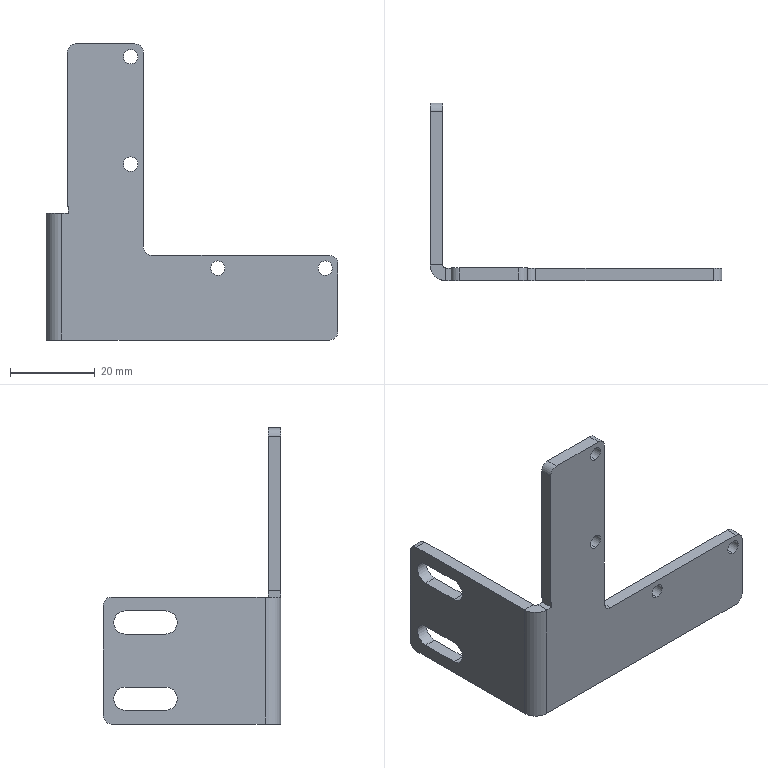Part | SolidWorks | features HoleWzd 2, EdgeFlange 1, Fillet 1, FlatPattern 1, SMBaseFlange 1, SheetMetal 1 | 1 solid | 43 faces | box 69 x 42 x 70 mm | volume 9835 mm3 | plane 22 | cylinder 21 | commonest cylinder face diameters 3.4 x8 4 x7 5.5 x4 1.473 x1 7.473 x1
STEP:
#1=CARTESIAN_POINT('',(15.,-3.,-30.1));
#2=VERTEX_POINT('',#1);
#3=CARTESIAN_POINT('',(15.,-3.,-26.7));
#4=VERTEX_POINT('',#3);
#5=CARTESIAN_POINT('',(15.,-3.,-28.4));
#6=DIRECTION('',(0.,1.,0.));
#7=DIRECTION('',(0.,0.,1.));
#8=AXIS2_PLACEMENT_3D('',#5,#6,#7);
#9=CIRCLE('',#8,1.7);
#10=EDGE_CURVE('',#2,#4,#9,.T.);
#11=ORIENTED_EDGE('',*,*,#10,.F.);
#12=CARTESIAN_POINT('',(15.,0.,-30.1));
#13=VERTEX_POINT('',#12);
#14=CARTESIAN_POINT('',(15.,0.,-30.1));
#15=DIRECTION('',(0.,1.,0.));
#16=VECTOR('',#15,1000.);
#17=LINE('',#14,#16);
#18=EDGE_CURVE('',#2,#13,#17,.T.);
#19=ORIENTED_EDGE('',*,*,#18,.T.);
#20=CARTESIAN_POINT('',(15.,0.,-26.7));
#21=VERTEX_POINT('',#20);
#22=CARTESIAN_POINT('',(15.,0.,-28.4));
#23=DIRECTION('',(0.,1.,0.));
#24=DIRECTION('',(0.,0.,1.));
#25=AXIS2_PLACEMENT_3D('',#22,#23,#24);
#26=CIRCLE('',#25,1.7);
#27=EDGE_CURVE('',#13,#21,#26,.T.);
#28=ORIENTED_EDGE('',*,*,#27,.T.);
#29=CARTESIAN_POINT('',(15.,0.,-26.7));
#30=DIRECTION('',(0.,1.,0.));
#31=VECTOR('',#30,1000.);
#32=LINE('',#29,#31);
#33=EDGE_CURVE('',#4,#21,#32,.T.);
#34=ORIENTED_EDGE('',*,*,#33,.F.);
#35=EDGE_LOOP('',(#11,#19,#28,#34));
#36=FACE_OUTER_BOUND('',#35,.T.);
#37=CARTESIAN_POINT('',(15.,0.,-28.4));
#38=DIRECTION('',(0.,1.,0.));
#39=DIRECTION('',(0.,0.,1.));
#40=AXIS2_PLACEMENT_3D('',#37,#38,#39);
#41=CYLINDRICAL_SURFACE('',#40,1.7);
#42=ADVANCED_FACE('',(#36),#41,.F.);
#43=CARTESIAN_POINT('',(15.,-3.,-4.7));
#44=VERTEX_POINT('',#43);
#45=CARTESIAN_POINT('',(15.,-3.,-1.3));
#46=VERTEX_POINT('',#45);
#47=CARTESIAN_POINT('',(15.,-3.,-3.));
#48=DIRECTION('',(0.,1.,0.));
#49=DIRECTION('',(0.,0.,1.));
#50=AXIS2_PLACEMENT_3D('',#47,#48,#49);
#51=CIRCLE('',#50,1.7);
#52=EDGE_CURVE('',#44,#46,#51,.T.);
#53=ORIENTED_EDGE('',*,*,#52,.F.);
#54=CARTESIAN_POINT('',(15.,0.,-4.7));
#55=VERTEX_POINT('',#54);
#56=CARTESIAN_POINT('',(15.,0.,-4.7));
#57=DIRECTION('',(0.,1.,0.));
#58=VECTOR('',#57,1000.);
#59=LINE('',#56,#58);
#60=EDGE_CURVE('',#44,#55,#59,.T.);
#61=ORIENTED_EDGE('',*,*,#60,.T.);
#62=CARTESIAN_POINT('',(15.,0.,-1.3));
#63=VERTEX_POINT('',#62);
#64=CARTESIAN_POINT('',(15.,0.,-3.));
#65=DIRECTION('',(0.,1.,0.));
#66=DIRECTION('',(0.,0.,1.));
#67=AXIS2_PLACEMENT_3D('',#64,#65,#66);
#68=CIRCLE('',#67,1.7);
#69=EDGE_CURVE('',#55,#63,#68,.T.);
#70=ORIENTED_EDGE('',*,*,#69,.T.);
#71=CARTESIAN_POINT('',(15.,0.,-1.3));
#72=DIRECTION('',(0.,1.,0.));
#73=VECTOR('',#72,1000.);
#74=LINE('',#71,#73);
#75=EDGE_CURVE('',#46,#63,#74,.T.);
#76=ORIENTED_EDGE('',*,*,#75,.F.);
#77=EDGE_LOOP('',(#53,#61,#70,#76));
#78=FACE_OUTER_BOUND('',#77,.T.);
#79=CARTESIAN_POINT('',(15.,0.,-3.));
#80=DIRECTION('',(0.,1.,0.));
#81=DIRECTION('',(0.,0.,1.));
#82=AXIS2_PLACEMENT_3D('',#79,#80,#81);
#83=CYLINDRICAL_SURFACE('',#82,1.7);
#84=ADVANCED_FACE('',(#78),#83,.F.);
#85=CARTESIAN_POINT('',(35.6,-3.,-54.7));
#86=VERTEX_POINT('',#85);
#87=CARTESIAN_POINT('',(35.6,-3.,-51.3));
#88=VERTEX_POINT('',#87);
#89=CARTESIAN_POINT('',(35.6,-3.,-53.));
#90=DIRECTION('',(0.,1.,0.));
#91=DIRECTION('',(0.,0.,1.));
#92=AXIS2_PLACEMENT_3D('',#89,#90,#91);
#93=CIRCLE('',#92,1.7);
#94=EDGE_CURVE('',#86,#88,#93,.T.);
#95=ORIENTED_EDGE('',*,*,#94,.F.);
#96=CARTESIAN_POINT('',(35.6,0.,-54.7));
#97=VERTEX_POINT('',#96);
#98=CARTESIAN_POINT('',(35.6,0.,-54.7));
#99=DIRECTION('',(0.,1.,0.));
#100=VECTOR('',#99,1000.);
#101=LINE('',#98,#100);
#102=EDGE_CURVE('',#86,#97,#101,.T.);
#103=ORIENTED_EDGE('',*,*,#102,.T.);
#104=CARTESIAN_POINT('',(35.6,0.,-51.3));
#105=VERTEX_POINT('',#104);
#106=CARTESIAN_POINT('',(35.6,0.,-53.));
#107=DIRECTION('',(0.,1.,0.));
#108=DIRECTION('',(0.,0.,1.));
#109=AXIS2_PLACEMENT_3D('',#106,#107,#108);
#110=CIRCLE('',#109,1.7);
#111=EDGE_CURVE('',#97,#105,#110,.T.);
#112=ORIENTED_EDGE('',*,*,#111,.T.);
#113=CARTESIAN_POINT('',(35.6,0.,-51.3));
#114=DIRECTION('',(0.,1.,0.));
#115=VECTOR('',#114,1000.);
#116=LINE('',#113,#115);
#117=EDGE_CURVE('',#88,#105,#116,.T.);
#118=ORIENTED_EDGE('',*,*,#117,.F.);
#119=EDGE_LOOP('',(#95,#103,#112,#118));
#120=FACE_OUTER_BOUND('',#119,.T.);
#121=CARTESIAN_POINT('',(35.6,0.,-53.));
#122=DIRECTION('',(0.,1.,0.));
#123=DIRECTION('',(0.,0.,1.));
#124=AXIS2_PLACEMENT_3D('',#121,#122,#123);
#125=CYLINDRICAL_SURFACE('',#124,1.7);
#126=ADVANCED_FACE('',(#120),#125,.F.);
#127=CARTESIAN_POINT('',(61.,-3.,-54.7));
#128=VERTEX_POINT('',#127);
#129=CARTESIAN_POINT('',(61.,-3.,-51.3));
#130=VERTEX_POINT('',#129);
#131=CARTESIAN_POINT('',(61.,-3.,-53.));
#132=DIRECTION('',(0.,1.,0.));
#133=DIRECTION('',(0.,0.,1.));
#134=AXIS2_PLACEMENT_3D('',#131,#132,#133);
#135=CIRCLE('',#134,1.7);
#136=EDGE_CURVE('',#128,#130,#135,.T.);
#137=ORIENTED_EDGE('',*,*,#136,.F.);
#138=CARTESIAN_POINT('',(61.,0.,-54.7));
#139=VERTEX_POINT('',#138);
#140=CARTESIAN_POINT('',(61.,0.,-54.7));
#141=DIRECTION('',(0.,1.,0.));
#142=VECTOR('',#141,1000.);
#143=LINE('',#140,#142);
#144=EDGE_CURVE('',#128,#139,#143,.T.);
#145=ORIENTED_EDGE('',*,*,#144,.T.);
#146=CARTESIAN_POINT('',(61.,0.,-51.3));
#147=VERTEX_POINT('',#146);
#148=CARTESIAN_POINT('',(61.,0.,-53.));
#149=DIRECTION('',(0.,1.,0.));
#150=DIRECTION('',(0.,0.,1.));
#151=AXIS2_PLACEMENT_3D('',#148,#149,#150);
#152=CIRCLE('',#151,1.7);
#153=EDGE_CURVE('',#139,#147,#152,.T.);
#154=ORIENTED_EDGE('',*,*,#153,.T.);
#155=CARTESIAN_POINT('',(61.,0.,-51.3));
#156=DIRECTION('',(0.,1.,0.));
#157=VECTOR('',#156,1000.);
#158=LINE('',#155,#157);
#159=EDGE_CURVE('',#130,#147,#158,.T.);
#160=ORIENTED_EDGE('',*,*,#159,.F.);
#161=EDGE_LOOP('',(#137,#145,#154,#160));
#162=FACE_OUTER_BOUND('',#161,.T.);
#163=CARTESIAN_POINT('',(61.,0.,-53.));
#164=DIRECTION('',(0.,1.,0.));
#165=DIRECTION('',(0.,0.,1.));
#166=AXIS2_PLACEMENT_3D('',#163,#164,#165);
#167=CYLINDRICAL_SURFACE('',#166,1.7);
#168=ADVANCED_FACE('',(#162),#167,.F.);
#169=CARTESIAN_POINT('',(-5.,24.25,-43.25));
#170=VERTEX_POINT('',#169);
#171=CARTESIAN_POINT('',(-5.,33.75,-43.25));
#172=VERTEX_POINT('',#171);
#173=CARTESIAN_POINT('',(-5.,24.25,-43.25));
#174=DIRECTION('',(0.,1.,0.));
#175=VECTOR('',#174,1000.);
#176=LINE('',#173,#175);
#177=EDGE_CURVE('',#170,#172,#176,.T.);
#178=ORIENTED_EDGE('',*,*,#177,.F.);
#179=CARTESIAN_POINT('',(-5.,24.25,-48.75));
#180=VERTEX_POINT('',#179);
#181=CARTESIAN_POINT('',(-5.,24.25,-46.));
#182=DIRECTION('',(-1.,0.,0.));
#183=DIRECTION('',(0.,0.,1.));
#184=AXIS2_PLACEMENT_3D('',#181,#182,#183);
#185=CIRCLE('',#184,2.75);
#186=EDGE_CURVE('',#180,#170,#185,.T.);
#187=ORIENTED_EDGE('',*,*,#186,.F.);
#188=CARTESIAN_POINT('',(-5.,33.75,-48.75));
#189=VERTEX_POINT('',#188);
#190=CARTESIAN_POINT('',(-5.,24.25,-48.75));
#191=DIRECTION('',(0.,1.,0.));
#192=VECTOR('',#191,1000.);
#193=LINE('',#190,#192);
#194=EDGE_CURVE('',#180,#189,#193,.T.);
#195=ORIENTED_EDGE('',*,*,#194,.T.);
#196=CARTESIAN_POINT('',(-5.,33.75,-46.));
#197=DIRECTION('',(-1.,0.,0.));
#198=DIRECTION('',(0.,0.,1.));
#199=AXIS2_PLACEMENT_3D('',#196,#197,#198);
#200=CIRCLE('',#199,2.75);
#201=EDGE_CURVE('',#172,#189,#200,.T.);
#202=ORIENTED_EDGE('',*,*,#201,.F.);
#203=EDGE_LOOP('',(#178,#187,#195,#202));
#204=FACE_BOUND('',#203,.T.);
#205=CARTESIAN_POINT('',(-5.,39.,-42.));
#206=VERTEX_POINT('',#205);
#207=CARTESIAN_POINT('',(-5.,39.,-68.));
#208=VERTEX_POINT('',#207);
#209=CARTESIAN_POINT('',(-5.,39.,-70.));
#210=DIRECTION('',(0.,0.,-1.));
#211=VECTOR('',#210,1000.);
#212=LINE('',#209,#211);
#213=EDGE_CURVE('',#206,#208,#212,.T.);
#214=ORIENTED_EDGE('',*,*,#213,.T.);
#215=CARTESIAN_POINT('',(-5.,37.,-70.));
#216=VERTEX_POINT('',#215);
#217=CARTESIAN_POINT('',(-5.,37.,-68.));
#218=DIRECTION('',(-1.,0.,0.));
#219=DIRECTION('',(0.,1.,0.));
#220=AXIS2_PLACEMENT_3D('',#217,#218,#219);
#221=CIRCLE('',#220,2.);
#222=EDGE_CURVE('',#208,#216,#221,.T.);
#223=ORIENTED_EDGE('',*,*,#222,.T.);
#224=CARTESIAN_POINT('',(-5.,0.7366,-70.));
#225=VERTEX_POINT('',#224);
#226=CARTESIAN_POINT('',(-5.,0.,-70.));
#227=DIRECTION('',(0.,-1.,0.));
#228=VECTOR('',#227,1000.);
#229=LINE('',#226,#228);
#230=EDGE_CURVE('',#216,#225,#229,.T.);
#231=ORIENTED_EDGE('',*,*,#230,.T.);
#232=CARTESIAN_POINT('',(-5.,0.7366,-40.));
#233=VERTEX_POINT('',#232);
#234=CARTESIAN_POINT('',(-5.,0.7366,0.));
#235=DIRECTION('',(0.,0.,-1.));
#236=VECTOR('',#235,1000.);
#237=LINE('',#234,#236);
#238=EDGE_CURVE('',#233,#225,#237,.T.);
#239=ORIENTED_EDGE('',*,*,#238,.F.);
#240=CARTESIAN_POINT('',(-5.,37.,-40.));
#241=VERTEX_POINT('',#240);
#242=CARTESIAN_POINT('',(-5.,39.,-40.));
#243=DIRECTION('',(0.,1.,0.));
#244=VECTOR('',#243,1000.);
#245=LINE('',#242,#244);
#246=EDGE_CURVE('',#233,#241,#245,.T.);
#247=ORIENTED_EDGE('',*,*,#246,.T.);
#248=CARTESIAN_POINT('',(-5.,37.,-42.));
#249=DIRECTION('',(-1.,0.,0.));
#250=DIRECTION('',(0.,1.,0.));
#251=AXIS2_PLACEMENT_3D('',#248,#249,#250);
#252=CIRCLE('',#251,2.);
#253=EDGE_CURVE('',#241,#206,#252,.T.);
#254=ORIENTED_EDGE('',*,*,#253,.T.);
#255=EDGE_LOOP('',(#214,#223,#231,#239,#247,#254));
#256=FACE_OUTER_BOUND('',#255,.T.);
#257=CARTESIAN_POINT('',(-5.,24.25,-61.25));
#258=VERTEX_POINT('',#257);
#259=CARTESIAN_POINT('',(-5.,33.75,-61.25));
#260=VERTEX_POINT('',#259);
#261=CARTESIAN_POINT('',(-5.,24.25,-61.25));
#262=DIRECTION('',(0.,1.,0.));
#263=VECTOR('',#262,1000.);
#264=LINE('',#261,#263);
#265=EDGE_CURVE('',#258,#260,#264,.T.);
#266=ORIENTED_EDGE('',*,*,#265,.F.);
#267=CARTESIAN_POINT('',(-5.,24.25,-66.75));
#268=VERTEX_POINT('',#267);
#269=CARTESIAN_POINT('',(-5.,24.25,-64.));
#270=DIRECTION('',(-1.,0.,0.));
#271=DIRECTION('',(0.,0.,1.));
#272=AXIS2_PLACEMENT_3D('',#269,#270,#271);
#273=CIRCLE('',#272,2.75);
#274=EDGE_CURVE('',#268,#258,#273,.T.);
#275=ORIENTED_EDGE('',*,*,#274,.F.);
#276=CARTESIAN_POINT('',(-5.,33.75,-66.75));
#277=VERTEX_POINT('',#276);
#278=CARTESIAN_POINT('',(-5.,24.25,-66.75));
#279=DIRECTION('',(0.,1.,0.));
#280=VECTOR('',#279,1000.);
#281=LINE('',#278,#280);
#282=EDGE_CURVE('',#268,#277,#281,.T.);
#283=ORIENTED_EDGE('',*,*,#282,.T.);
#284=CARTESIAN_POINT('',(-5.,33.75,-64.));
#285=DIRECTION('',(-1.,0.,0.));
#286=DIRECTION('',(0.,0.,1.));
#287=AXIS2_PLACEMENT_3D('',#284,#285,#286);
#288=CIRCLE('',#287,2.75);
#289=EDGE_CURVE('',#260,#277,#288,.T.);
#290=ORIENTED_EDGE('',*,*,#289,.F.);
#291=EDGE_LOOP('',(#266,#275,#283,#290));
#292=FACE_BOUND('',#291,.T.);
#293=CARTESIAN_POINT('',(-5.,0.,0.));
#294=DIRECTION('',(1.,0.,0.));
#295=DIRECTION('',(0.,1.,0.));
#296=AXIS2_PLACEMENT_3D('',#293,#294,#295);
#297=PLANE('',#296);
#298=ADVANCED_FACE('',(#204,#256,#292),#297,.F.);
#299=CARTESIAN_POINT('',(0.,-3.,-38.5));
#300=VERTEX_POINT('',#299);
#301=CARTESIAN_POINT('',(0.,-3.,-2.));
#302=VERTEX_POINT('',#301);
#303=CARTESIAN_POINT('',(0.,-3.,-40.));
#304=DIRECTION('',(0.,0.,1.));
#305=VECTOR('',#304,1000.);
#306=LINE('',#303,#305);
#307=EDGE_CURVE('',#300,#302,#306,.T.);
#308=ORIENTED_EDGE('',*,*,#307,.T.);
#309=CARTESIAN_POINT('',(0.,0.,-2.));
#310=VERTEX_POINT('',#309);
#311=CARTESIAN_POINT('',(0.,-3.,-2.));
#312=DIRECTION('',(0.,1.,0.));
#313=VECTOR('',#312,1000.);
#314=LINE('',#311,#313);
#315=EDGE_CURVE('',#302,#310,#314,.T.);
#316=ORIENTED_EDGE('',*,*,#315,.T.);
#317=CARTESIAN_POINT('',(0.,0.,-38.5));
#318=VERTEX_POINT('',#317);
#319=CARTESIAN_POINT('',(0.,0.,-40.));
#320=DIRECTION('',(0.,0.,1.));
#321=VECTOR('',#320,1000.);
#322=LINE('',#319,#321);
#323=EDGE_CURVE('',#318,#310,#322,.T.);
#324=ORIENTED_EDGE('',*,*,#323,.F.);
#325=CARTESIAN_POINT('',(0.,-3.,-38.5));
#326=DIRECTION('',(0.,-1.,0.));
#327=VECTOR('',#326,1000.);
#328=LINE('',#325,#327);
#329=EDGE_CURVE('',#318,#300,#328,.T.);
#330=ORIENTED_EDGE('',*,*,#329,.T.);
#331=EDGE_LOOP('',(#308,#316,#324,#330));
#332=FACE_OUTER_BOUND('',#331,.T.);
#333=CARTESIAN_POINT('',(0.,-3.,-40.));
#334=DIRECTION('',(-1.,0.,0.));
#335=DIRECTION('',(0.,0.,1.));
#336=AXIS2_PLACEMENT_3D('',#333,#334,#335);
#337=PLANE('',#336);
#338=ADVANCED_FACE('',(#332),#337,.T.);
#339=CARTESIAN_POINT('',(-1.263,0.,-40.));
#340=VERTEX_POINT('',#339);
#341=CARTESIAN_POINT('',(0.2366,0.,-40.));
#342=VERTEX_POINT('',#341);
#343=CARTESIAN_POINT('',(-2.,0.,-40.));
#344=DIRECTION('',(1.,0.,0.));
#345=VECTOR('',#344,1000.);
#346=LINE('',#343,#345);
#347=EDGE_CURVE('',#340,#342,#346,.T.);
#348=ORIENTED_EDGE('',*,*,#347,.F.);
#349=CARTESIAN_POINT('',(-1.263,-3.,-40.));
#350=VERTEX_POINT('',#349);
#351=CARTESIAN_POINT('',(-1.263,0.,-40.));
#352=DIRECTION('',(0.,-1.,0.));
#353=VECTOR('',#352,1000.);
#354=LINE('',#351,#353);
#355=EDGE_CURVE('',#340,#350,#354,.T.);
#356=ORIENTED_EDGE('',*,*,#355,.T.);
#357=CARTESIAN_POINT('',(0.2366,-3.,-40.));
#358=VERTEX_POINT('',#357);
#359=CARTESIAN_POINT('',(-2.,-3.,-40.));
#360=DIRECTION('',(1.,0.,0.));
#361=VECTOR('',#360,1000.);
#362=LINE('',#359,#361);
#363=EDGE_CURVE('',#350,#358,#362,.T.);
#364=ORIENTED_EDGE('',*,*,#363,.T.);
#365=CARTESIAN_POINT('',(0.2366,0.,-40.));
#366=DIRECTION('',(0.,-1.,0.));
#367=VECTOR('',#366,1000.);
#368=LINE('',#365,#367);
#369=EDGE_CURVE('',#342,#358,#368,.T.);
#370=ORIENTED_EDGE('',*,*,#369,.F.);
#371=EDGE_LOOP('',(#348,#356,#364,#370));
#372=FACE_OUTER_BOUND('',#371,.T.);
#373=CARTESIAN_POINT('',(-2.,-3.,-40.));
#374=DIRECTION('',(0.,0.,1.));
#375=DIRECTION('',(1.,0.,0.));
#376=AXIS2_PLACEMENT_3D('',#373,#374,#375);
#377=PLANE('',#376);
#378=ADVANCED_FACE('',(#372),#377,.T.);
#379=CARTESIAN_POINT('',(15.,-3.,-28.4));
#380=DIRECTION('',(0.,1.,0.));
#381=DIRECTION('',(0.,0.,1.));
#382=AXIS2_PLACEMENT_3D('',#379,#380,#381);
#383=CIRCLE('',#382,1.7);
#384=EDGE_CURVE('',#4,#2,#383,.T.);
#385=ORIENTED_EDGE('',*,*,#384,.T.);
#386=ORIENTED_EDGE('',*,*,#10,.T.);
#387=EDGE_LOOP('',(#385,#386));
#388=FACE_BOUND('',#387,.T.);
#389=CARTESIAN_POINT('',(15.,-3.,-3.));
#390=DIRECTION('',(0.,1.,0.));
#391=DIRECTION('',(0.,0.,1.));
#392=AXIS2_PLACEMENT_3D('',#389,#390,#391);
#393=CIRCLE('',#392,1.7);
#394=EDGE_CURVE('',#46,#44,#393,.T.);
#395=ORIENTED_EDGE('',*,*,#394,.T.);
#396=ORIENTED_EDGE('',*,*,#52,.T.);
#397=EDGE_LOOP('',(#395,#396));
#398=FACE_BOUND('',#397,.T.);
#399=CARTESIAN_POINT('',(35.6,-3.,-53.));
#400=DIRECTION('',(0.,1.,0.));
#401=DIRECTION('',(0.,0.,1.));
#402=AXIS2_PLACEMENT_3D('',#399,#400,#401);
#403=CIRCLE('',#402,1.7);
#404=EDGE_CURVE('',#88,#86,#403,.T.);
#405=ORIENTED_EDGE('',*,*,#404,.T.);
#406=ORIENTED_EDGE('',*,*,#94,.T.);
#407=EDGE_LOOP('',(#405,#406));
#408=FACE_BOUND('',#407,.T.);
#409=CARTESIAN_POINT('',(61.,-3.,-53.));
#410=DIRECTION('',(0.,1.,0.));
#411=DIRECTION('',(0.,0.,1.));
#412=AXIS2_PLACEMENT_3D('',#409,#410,#411);
#413=CIRCLE('',#412,1.7);
#414=EDGE_CURVE('',#130,#128,#413,.T.);
#415=ORIENTED_EDGE('',*,*,#414,.T.);
#416=ORIENTED_EDGE('',*,*,#136,.T.);
#417=EDGE_LOOP('',(#415,#416));
#418=FACE_BOUND('',#417,.T.);
#419=CARTESIAN_POINT('',(62.,-3.,-70.));
#420=VERTEX_POINT('',#419);
#421=CARTESIAN_POINT('',(-1.263,-3.,-70.));
#422=VERTEX_POINT('',#421);
#423=CARTESIAN_POINT('',(64.,-3.,-70.));
#424=DIRECTION('',(-1.,0.,0.));
#425=VECTOR('',#424,1000.);
#426=LINE('',#423,#425);
#427=EDGE_CURVE('',#420,#422,#426,.T.);
#428=ORIENTED_EDGE('',*,*,#427,.F.);
#429=CARTESIAN_POINT('',(64.,-3.,-68.));
#430=VERTEX_POINT('',#429);
#431=CARTESIAN_POINT('',(62.,-3.,-68.));
#432=DIRECTION('',(0.,-1.,0.));
#433=DIRECTION('',(0.,0.,1.));
#434=AXIS2_PLACEMENT_3D('',#431,#432,#433);
#435=CIRCLE('',#434,2.);
#436=EDGE_CURVE('',#420,#430,#435,.T.);
#437=ORIENTED_EDGE('',*,*,#436,.T.);
#438=CARTESIAN_POINT('',(64.,-3.,-52.));
#439=VERTEX_POINT('',#438);
#440=CARTESIAN_POINT('',(64.,-3.,-50.));
#441=DIRECTION('',(0.,0.,-1.));
#442=VECTOR('',#441,1000.);
#443=LINE('',#440,#442);
#444=EDGE_CURVE('',#439,#430,#443,.T.);
#445=ORIENTED_EDGE('',*,*,#444,.F.);
#446=CARTESIAN_POINT('',(62.,-3.,-50.));
#447=VERTEX_POINT('',#446);
#448=CARTESIAN_POINT('',(62.,-3.,-52.));
#449=DIRECTION('',(0.,-1.,0.));
#450=DIRECTION('',(0.,0.,1.));
#451=AXIS2_PLACEMENT_3D('',#448,#449,#450);
#452=CIRCLE('',#451,2.);
#453=EDGE_CURVE('',#439,#447,#452,.T.);
#454=ORIENTED_EDGE('',*,*,#453,.T.);
#455=CARTESIAN_POINT('',(20.,-3.,-50.));
#456=VERTEX_POINT('',#455);
#457=CARTESIAN_POINT('',(18.,-3.,-50.));
#458=DIRECTION('',(1.,0.,0.));
#459=VECTOR('',#458,1000.);
#460=LINE('',#457,#459);
#461=EDGE_CURVE('',#456,#447,#460,.T.);
#462=ORIENTED_EDGE('',*,*,#461,.F.);
#463=CARTESIAN_POINT('',(18.,-3.,-48.));
#464=VERTEX_POINT('',#463);
#465=CARTESIAN_POINT('',(20.,-3.,-48.));
#466=DIRECTION('',(0.,1.,0.));
#467=DIRECTION('',(0.,0.,1.));
#468=AXIS2_PLACEMENT_3D('',#465,#466,#467);
#469=CIRCLE('',#468,2.);
#470=EDGE_CURVE('',#456,#464,#469,.T.);
#471=ORIENTED_EDGE('',*,*,#470,.T.);
#472=CARTESIAN_POINT('',(18.,-3.,-2.));
#473=VERTEX_POINT('',#472);
#474=CARTESIAN_POINT('',(18.,-3.,0.));
#475=DIRECTION('',(0.,0.,-1.));
#476=VECTOR('',#475,1000.);
#477=LINE('',#474,#476);
#478=EDGE_CURVE('',#473,#464,#477,.T.);
#479=ORIENTED_EDGE('',*,*,#478,.F.);
#480=CARTESIAN_POINT('',(16.,-3.,0.));
#481=VERTEX_POINT('',#480);
#482=CARTESIAN_POINT('',(16.,-3.,-2.));
#483=DIRECTION('',(0.,-1.,0.));
#484=DIRECTION('',(0.,0.,1.));
#485=AXIS2_PLACEMENT_3D('',#482,#483,#484);
#486=CIRCLE('',#485,2.);
#487=EDGE_CURVE('',#473,#481,#486,.T.);
#488=ORIENTED_EDGE('',*,*,#487,.T.);
#489=CARTESIAN_POINT('',(2.,-3.,0.));
#490=VERTEX_POINT('',#489);
#491=CARTESIAN_POINT('',(0.,-3.,0.));
#492=DIRECTION('',(1.,0.,0.));
#493=VECTOR('',#492,1000.);
#494=LINE('',#491,#493);
#495=EDGE_CURVE('',#490,#481,#494,.T.);
#496=ORIENTED_EDGE('',*,*,#495,.F.);
#497=CARTESIAN_POINT('',(2.,-3.,-2.));
#498=DIRECTION('',(0.,-1.,0.));
#499=DIRECTION('',(0.,0.,1.));
#500=AXIS2_PLACEMENT_3D('',#497,#498,#499);
#501=CIRCLE('',#500,2.);
#502=EDGE_CURVE('',#490,#302,#501,.T.);
#503=ORIENTED_EDGE('',*,*,#502,.T.);
#504=ORIENTED_EDGE('',*,*,#307,.F.);
#505=CARTESIAN_POINT('',(0.2366,-3.,-38.5));
#506=VERTEX_POINT('',#505);
#507=CARTESIAN_POINT('',(0.,-3.,-38.5));
#508=DIRECTION('',(-1.,0.,0.));
#509=VECTOR('',#508,1000.);
#510=LINE('',#507,#509);
#511=EDGE_CURVE('',#506,#300,#510,.T.);
#512=ORIENTED_EDGE('',*,*,#511,.F.);
#513=CARTESIAN_POINT('',(0.2366,-3.,0.));
#514=DIRECTION('',(0.,0.,1.));
#515=VECTOR('',#514,1000.);
#516=LINE('',#513,#515);
#517=EDGE_CURVE('',#358,#506,#516,.T.);
#518=ORIENTED_EDGE('',*,*,#517,.F.);
#519=ORIENTED_EDGE('',*,*,#363,.F.);
#520=CARTESIAN_POINT('',(-1.263,-3.,-40.));
#521=DIRECTION('',(0.,0.,-1.));
#522=VECTOR('',#521,1000.);
#523=LINE('',#520,#522);
#524=EDGE_CURVE('',#350,#422,#523,.T.);
#525=ORIENTED_EDGE('',*,*,#524,.T.);
#526=EDGE_LOOP('',(#428,#437,#445,#454,#462,#471,#479,#488,#496,#503,#504,#512,#518,#519,#525));
#527=FACE_OUTER_BOUND('',#526,.T.);
#528=CARTESIAN_POINT('',(0.,-3.,0.));
#529=DIRECTION('',(0.,1.,0.));
#530=DIRECTION('',(0.,0.,1.));
#531=AXIS2_PLACEMENT_3D('',#528,#529,#530);
#532=PLANE('',#531);
#533=ADVANCED_FACE('',(#388,#398,#408,#418,#527),#532,.F.);
#534=CARTESIAN_POINT('',(15.,0.,-28.4));
#535=DIRECTION('',(0.,1.,0.));
#536=DIRECTION('',(0.,0.,1.));
#537=AXIS2_PLACEMENT_3D('',#534,#535,#536);
#538=CIRCLE('',#537,1.7);
#539=EDGE_CURVE('',#21,#13,#538,.T.);
#540=ORIENTED_EDGE('',*,*,#539,.F.);
#541=ORIENTED_EDGE('',*,*,#27,.F.);
#542=EDGE_LOOP('',(#540,#541));
#543=FACE_BOUND('',#542,.T.);
#544=CARTESIAN_POINT('',(15.,0.,-3.));
#545=DIRECTION('',(0.,1.,0.));
#546=DIRECTION('',(0.,0.,1.));
#547=AXIS2_PLACEMENT_3D('',#544,#545,#546);
#548=CIRCLE('',#547,1.7);
#549=EDGE_CURVE('',#63,#55,#548,.T.);
#550=ORIENTED_EDGE('',*,*,#549,.F.);
#551=ORIENTED_EDGE('',*,*,#69,.F.);
#552=EDGE_LOOP('',(#550,#551));
#553=FACE_BOUND('',#552,.T.);
#554=CARTESIAN_POINT('',(35.6,0.,-53.));
#555=DIRECTION('',(0.,1.,0.));
#556=DIRECTION('',(0.,0.,1.));
#557=AXIS2_PLACEMENT_3D('',#554,#555,#556);
#558=CIRCLE('',#557,1.7);
#559=EDGE_CURVE('',#105,#97,#558,.T.);
#560=ORIENTED_EDGE('',*,*,#559,.F.);
#561=ORIENTED_EDGE('',*,*,#111,.F.);
#562=EDGE_LOOP('',(#560,#561));
#563=FACE_BOUND('',#562,.T.);
#564=CARTESIAN_POINT('',(61.,0.,-53.));
#565=DIRECTION('',(0.,1.,0.));
#566=DIRECTION('',(0.,0.,1.));
#567=AXIS2_PLACEMENT_3D('',#564,#565,#566);
#568=CIRCLE('',#567,1.7);
#569=EDGE_CURVE('',#147,#139,#568,.T.);
#570=ORIENTED_EDGE('',*,*,#569,.F.);
#571=ORIENTED_EDGE('',*,*,#153,.F.);
#572=EDGE_LOOP('',(#570,#571));
#573=FACE_BOUND('',#572,.T.);
#574=CARTESIAN_POINT('',(64.,0.,-52.));
#575=VERTEX_POINT('',#574);
#576=CARTESIAN_POINT('',(64.,0.,-68.));
#577=VERTEX_POINT('',#576);
#578=CARTESIAN_POINT('',(64.,0.,-50.));
#579=DIRECTION('',(0.,0.,-1.));
#580=VECTOR('',#579,1000.);
#581=LINE('',#578,#580);
#582=EDGE_CURVE('',#575,#577,#581,.T.);
#583=ORIENTED_EDGE('',*,*,#582,.T.);
#584=CARTESIAN_POINT('',(62.,0.,-70.));
#585=VERTEX_POINT('',#584);
#586=CARTESIAN_POINT('',(62.,0.,-68.));
#587=DIRECTION('',(0.,1.,0.));
#588=DIRECTION('',(0.,0.,1.));
#589=AXIS2_PLACEMENT_3D('',#586,#587,#588);
#590=CIRCLE('',#589,2.);
#591=EDGE_CURVE('',#577,#585,#590,.T.);
#592=ORIENTED_EDGE('',*,*,#591,.T.);
#593=CARTESIAN_POINT('',(-1.263,0.,-70.));
#594=VERTEX_POINT('',#593);
#595=CARTESIAN_POINT('',(64.,0.,-70.));
#596=DIRECTION('',(-1.,0.,0.));
#597=VECTOR('',#596,1000.);
#598=LINE('',#595,#597);
#599=EDGE_CURVE('',#585,#594,#598,.T.);
#600=ORIENTED_EDGE('',*,*,#599,.T.);
#601=CARTESIAN_POINT('',(-1.263,0.,-40.));
#602=DIRECTION('',(0.,0.,-1.));
#603=VECTOR('',#602,1000.);
#604=LINE('',#601,#603);
#605=EDGE_CURVE('',#340,#594,#604,.T.);
#606=ORIENTED_EDGE('',*,*,#605,.F.);
#607=ORIENTED_EDGE('',*,*,#347,.T.);
#608=CARTESIAN_POINT('',(0.2366,0.,-38.5));
#609=VERTEX_POINT('',#608);
#610=CARTESIAN_POINT('',(0.2366,0.,-38.5));
#611=DIRECTION('',(0.,0.,-1.));
#612=VECTOR('',#611,1000.);
#613=LINE('',#610,#612);
#614=EDGE_CURVE('',#609,#342,#613,.T.);
#615=ORIENTED_EDGE('',*,*,#614,.F.);
#616=CARTESIAN_POINT('',(0.,0.,-38.5));
#617=DIRECTION('',(-1.,0.,0.));
#618=VECTOR('',#617,1000.);
#619=LINE('',#616,#618);
#620=EDGE_CURVE('',#609,#318,#619,.T.);
#621=ORIENTED_EDGE('',*,*,#620,.T.);
#622=ORIENTED_EDGE('',*,*,#323,.T.);
#623=CARTESIAN_POINT('',(2.,0.,0.));
#624=VERTEX_POINT('',#623);
#625=CARTESIAN_POINT('',(2.,0.,-2.));
#626=DIRECTION('',(0.,1.,0.));
#627=DIRECTION('',(0.,0.,1.));
#628=AXIS2_PLACEMENT_3D('',#625,#626,#627);
#629=CIRCLE('',#628,2.);
#630=EDGE_CURVE('',#310,#624,#629,.T.);
#631=ORIENTED_EDGE('',*,*,#630,.T.);
#632=CARTESIAN_POINT('',(16.,0.,0.));
#633=VERTEX_POINT('',#632);
#634=CARTESIAN_POINT('',(0.,0.,0.));
#635=DIRECTION('',(1.,0.,0.));
#636=VECTOR('',#635,1000.);
#637=LINE('',#634,#636);
#638=EDGE_CURVE('',#624,#633,#637,.T.);
#639=ORIENTED_EDGE('',*,*,#638,.T.);
#640=CARTESIAN_POINT('',(18.,0.,-2.));
#641=VERTEX_POINT('',#640);
#642=CARTESIAN_POINT('',(16.,0.,-2.));
#643=DIRECTION('',(0.,1.,0.));
#644=DIRECTION('',(0.,0.,1.));
#645=AXIS2_PLACEMENT_3D('',#642,#643,#644);
#646=CIRCLE('',#645,2.);
#647=EDGE_CURVE('',#633,#641,#646,.T.);
#648=ORIENTED_EDGE('',*,*,#647,.T.);
#649=CARTESIAN_POINT('',(18.,0.,-48.));
#650=VERTEX_POINT('',#649);
#651=CARTESIAN_POINT('',(18.,0.,0.));
#652=DIRECTION('',(0.,0.,-1.));
#653=VECTOR('',#652,1000.);
#654=LINE('',#651,#653);
#655=EDGE_CURVE('',#641,#650,#654,.T.);
#656=ORIENTED_EDGE('',*,*,#655,.T.);
#657=CARTESIAN_POINT('',(20.,0.,-50.));
#658=VERTEX_POINT('',#657);
#659=CARTESIAN_POINT('',(20.,0.,-48.));
#660=DIRECTION('',(0.,-1.,0.));
#661=DIRECTION('',(0.,0.,1.));
#662=AXIS2_PLACEMENT_3D('',#659,#660,#661);
#663=CIRCLE('',#662,2.);
#664=EDGE_CURVE('',#650,#658,#663,.T.);
#665=ORIENTED_EDGE('',*,*,#664,.T.);
#666=CARTESIAN_POINT('',(62.,0.,-50.));
#667=VERTEX_POINT('',#666);
#668=CARTESIAN_POINT('',(18.,0.,-50.));
#669=DIRECTION('',(1.,0.,0.));
#670=VECTOR('',#669,1000.);
#671=LINE('',#668,#670);
#672=EDGE_CURVE('',#658,#667,#671,.T.);
#673=ORIENTED_EDGE('',*,*,#672,.T.);
#674=CARTESIAN_POINT('',(62.,0.,-52.));
#675=DIRECTION('',(0.,1.,0.));
#676=DIRECTION('',(0.,0.,1.));
#677=AXIS2_PLACEMENT_3D('',#674,#675,#676);
#678=CIRCLE('',#677,2.);
#679=EDGE_CURVE('',#667,#575,#678,.T.);
#680=ORIENTED_EDGE('',*,*,#679,.T.);
#681=EDGE_LOOP('',(#583,#592,#600,#606,#607,#615,#621,#622,#631,#639,#648,#656,#665,#673,#680));
#682=FACE_OUTER_BOUND('',#681,.T.);
#683=CARTESIAN_POINT('',(0.,0.,0.));
#684=DIRECTION('',(0.,1.,0.));
#685=DIRECTION('',(0.,0.,1.));
#686=AXIS2_PLACEMENT_3D('',#683,#684,#685);
#687=PLANE('',#686);
#688=ADVANCED_FACE('',(#543,#553,#563,#573,#682),#687,.T.);
#689=ORIENTED_EDGE('',*,*,#599,.F.);
#690=CARTESIAN_POINT('',(62.,-3.,-70.));
#691=DIRECTION('',(0.,-1.,0.));
#692=VECTOR('',#691,1000.);
#693=LINE('',#690,#692);
#694=EDGE_CURVE('',#585,#420,#693,.T.);
#695=ORIENTED_EDGE('',*,*,#694,.T.);
#696=ORIENTED_EDGE('',*,*,#427,.T.);
#697=CARTESIAN_POINT('',(-1.263,0.,-70.));
#698=DIRECTION('',(0.,-1.,0.));
#699=VECTOR('',#698,1000.);
#700=LINE('',#697,#699);
#701=EDGE_CURVE('',#594,#422,#700,.T.);
#702=ORIENTED_EDGE('',*,*,#701,.F.);
#703=EDGE_LOOP('',(#689,#695,#696,#702));
#704=FACE_OUTER_BOUND('',#703,.T.);
#705=CARTESIAN_POINT('',(64.,-3.,-70.));
#706=DIRECTION('',(0.,0.,-1.));
#707=DIRECTION('',(-1.,0.,0.));
#708=AXIS2_PLACEMENT_3D('',#705,#706,#707);
#709=PLANE('',#708);
#710=ADVANCED_FACE('',(#704),#709,.T.);
#711=ORIENTED_EDGE('',*,*,#444,.T.);
#712=CARTESIAN_POINT('',(64.,-3.,-68.));
#713=DIRECTION('',(0.,1.,0.));
#714=VECTOR('',#713,1000.);
#715=LINE('',#712,#714);
#716=EDGE_CURVE('',#430,#577,#715,.T.);
#717=ORIENTED_EDGE('',*,*,#716,.T.);
#718=ORIENTED_EDGE('',*,*,#582,.F.);
#719=CARTESIAN_POINT('',(64.,-3.,-52.));
#720=DIRECTION('',(0.,-1.,0.));
#721=VECTOR('',#720,1000.);
#722=LINE('',#719,#721);
#723=EDGE_CURVE('',#575,#439,#722,.T.);
#724=ORIENTED_EDGE('',*,*,#723,.T.);
#725=EDGE_LOOP('',(#711,#717,#718,#724));
#726=FACE_OUTER_BOUND('',#725,.T.);
#727=CARTESIAN_POINT('',(64.,-3.,-50.));
#728=DIRECTION('',(1.,0.,0.));
#729=DIRECTION('',(0.,0.,-1.));
#730=AXIS2_PLACEMENT_3D('',#727,#728,#729);
#731=PLANE('',#730);
#732=ADVANCED_FACE('',(#726),#731,.T.);
#733=ORIENTED_EDGE('',*,*,#672,.F.);
#734=CARTESIAN_POINT('',(20.,-3.,-50.));
#735=DIRECTION('',(0.,-1.,0.));
#736=VECTOR('',#735,1000.);
#737=LINE('',#734,#736);
#738=EDGE_CURVE('',#658,#456,#737,.T.);
#739=ORIENTED_EDGE('',*,*,#738,.T.);
#740=ORIENTED_EDGE('',*,*,#461,.T.);
#741=CARTESIAN_POINT('',(62.,-3.,-50.));
#742=DIRECTION('',(0.,1.,0.));
#743=VECTOR('',#742,1000.);
#744=LINE('',#741,#743);
#745=EDGE_CURVE('',#447,#667,#744,.T.);
#746=ORIENTED_EDGE('',*,*,#745,.T.);
#747=EDGE_LOOP('',(#733,#739,#740,#746));
#748=FACE_OUTER_BOUND('',#747,.T.);
#749=CARTESIAN_POINT('',(18.,-3.,-50.));
#750=DIRECTION('',(0.,0.,1.));
#751=DIRECTION('',(1.,0.,0.));
#752=AXIS2_PLACEMENT_3D('',#749,#750,#751);
#753=PLANE('',#752);
#754=ADVANCED_FACE('',(#748),#753,.T.);
#755=ORIENTED_EDGE('',*,*,#478,.T.);
#756=CARTESIAN_POINT('',(18.,0.,-48.));
#757=DIRECTION('',(0.,1.,0.));
#758=VECTOR('',#757,1000.);
#759=LINE('',#756,#758);
#760=EDGE_CURVE('',#464,#650,#759,.T.);
#761=ORIENTED_EDGE('',*,*,#760,.T.);
#762=ORIENTED_EDGE('',*,*,#655,.F.);
#763=CARTESIAN_POINT('',(18.,-3.,-2.));
#764=DIRECTION('',(0.,-1.,0.));
#765=VECTOR('',#764,1000.);
#766=LINE('',#763,#765);
#767=EDGE_CURVE('',#641,#473,#766,.T.);
#768=ORIENTED_EDGE('',*,*,#767,.T.);
#769=EDGE_LOOP('',(#755,#761,#762,#768));
#770=FACE_OUTER_BOUND('',#769,.T.);
#771=CARTESIAN_POINT('',(18.,-3.,0.));
#772=DIRECTION('',(1.,0.,0.));
#773=DIRECTION('',(0.,0.,-1.));
#774=AXIS2_PLACEMENT_3D('',#771,#772,#773);
#775=PLANE('',#774);
#776=ADVANCED_FACE('',(#770),#775,.T.);
#777=ORIENTED_EDGE('',*,*,#495,.T.);
#778=CARTESIAN_POINT('',(16.,-3.,0.));
#779=DIRECTION('',(0.,1.,0.));
#780=VECTOR('',#779,1000.);
#781=LINE('',#778,#780);
#782=EDGE_CURVE('',#481,#633,#781,.T.);
#783=ORIENTED_EDGE('',*,*,#782,.T.);
#784=ORIENTED_EDGE('',*,*,#638,.F.);
#785=CARTESIAN_POINT('',(2.,-3.,0.));
#786=DIRECTION('',(0.,-1.,0.));
#787=VECTOR('',#786,1000.);
#788=LINE('',#785,#787);
#789=EDGE_CURVE('',#624,#490,#788,.T.);
#790=ORIENTED_EDGE('',*,*,#789,.T.);
#791=EDGE_LOOP('',(#777,#783,#784,#790));
#792=FACE_OUTER_BOUND('',#791,.T.);
#793=CARTESIAN_POINT('',(0.,-3.,0.));
#794=DIRECTION('',(0.,0.,1.));
#795=DIRECTION('',(1.,0.,0.));
#796=AXIS2_PLACEMENT_3D('',#793,#794,#795);
#797=PLANE('',#796);
#798=ADVANCED_FACE('',(#792),#797,.T.);
#799=ORIENTED_EDGE('',*,*,#369,.T.);
#800=ORIENTED_EDGE('',*,*,#517,.T.);
#801=CARTESIAN_POINT('',(0.2366,0.,-38.5));
#802=DIRECTION('',(0.,-1.,0.));
#803=VECTOR('',#802,1000.);
#804=LINE('',#801,#803);
#805=EDGE_CURVE('',#609,#506,#804,.T.);
#806=ORIENTED_EDGE('',*,*,#805,.F.);
#807=ORIENTED_EDGE('',*,*,#614,.T.);
#808=EDGE_LOOP('',(#799,#800,#806,#807));
#809=FACE_OUTER_BOUND('',#808,.T.);
#810=CARTESIAN_POINT('',(0.2366,0.,-38.5));
#811=DIRECTION('',(-1.,0.,0.));
#812=DIRECTION('',(0.,0.,1.));
#813=AXIS2_PLACEMENT_3D('',#810,#811,#812);
#814=PLANE('',#813);
#815=ADVANCED_FACE('',(#809),#814,.T.);
#816=ORIENTED_EDGE('',*,*,#329,.F.);
#817=ORIENTED_EDGE('',*,*,#620,.F.);
#818=ORIENTED_EDGE('',*,*,#805,.T.);
#819=ORIENTED_EDGE('',*,*,#511,.T.);
#820=EDGE_LOOP('',(#816,#817,#818,#819));
#821=FACE_OUTER_BOUND('',#820,.T.);
#822=CARTESIAN_POINT('',(-2.,0.,-38.5));
#823=DIRECTION('',(0.,0.,-1.));
#824=DIRECTION('',(0.,1.,0.));
#825=AXIS2_PLACEMENT_3D('',#822,#823,#824);
#826=PLANE('',#825);
#827=ADVANCED_FACE('',(#821),#826,.T.);
#828=CARTESIAN_POINT('',(-2.,0.7366,-70.));
#829=VERTEX_POINT('',#828);
#830=CARTESIAN_POINT('',(-2.,0.7366,-70.));
#831=DIRECTION('',(-1.,0.,0.));
#832=VECTOR('',#831,1000.);
#833=LINE('',#830,#832);
#834=EDGE_CURVE('',#829,#225,#833,.T.);
#835=ORIENTED_EDGE('',*,*,#834,.F.);
#836=CARTESIAN_POINT('',(-1.263,0.7366,-70.));
#837=DIRECTION('',(0.,0.,-1.));
#838=DIRECTION('',(1.,0.,0.));
#839=AXIS2_PLACEMENT_3D('',#836,#837,#838);
#840=CIRCLE('',#839,0.7366);
#841=EDGE_CURVE('',#594,#829,#840,.T.);
#842=ORIENTED_EDGE('',*,*,#841,.F.);
#843=ORIENTED_EDGE('',*,*,#701,.T.);
#844=CARTESIAN_POINT('',(-1.263,0.7366,-70.));
#845=DIRECTION('',(0.,0.,-1.));
#846=DIRECTION('',(1.,0.,0.));
#847=AXIS2_PLACEMENT_3D('',#844,#845,#846);
#848=CIRCLE('',#847,3.737);
#849=EDGE_CURVE('',#422,#225,#848,.T.);
#850=ORIENTED_EDGE('',*,*,#849,.T.);
#851=EDGE_LOOP('',(#835,#842,#843,#850));
#852=FACE_OUTER_BOUND('',#851,.T.);
#853=CARTESIAN_POINT('',(-1.263,0.7366,-70.));
#854=DIRECTION('',(0.,0.,-1.));
#855=DIRECTION('',(-1.,0.,0.));
#856=AXIS2_PLACEMENT_3D('',#853,#854,#855);
#857=PLANE('',#856);
#858=ADVANCED_FACE('',(#852),#857,.T.);
#859=CARTESIAN_POINT('',(-2.,0.7366,-40.));
#860=VERTEX_POINT('',#859);
#861=CARTESIAN_POINT('',(-1.263,0.7366,-40.));
#862=DIRECTION('',(0.,0.,1.));
#863=DIRECTION('',(1.,0.,0.));
#864=AXIS2_PLACEMENT_3D('',#861,#862,#863);
#865=CIRCLE('',#864,0.7366);
#866=EDGE_CURVE('',#860,#340,#865,.T.);
#867=ORIENTED_EDGE('',*,*,#866,.F.);
#868=CARTESIAN_POINT('',(-2.,0.7366,-40.));
#869=DIRECTION('',(-1.,0.,0.));
#870=VECTOR('',#869,1000.);
#871=LINE('',#868,#870);
#872=EDGE_CURVE('',#860,#233,#871,.T.);
#873=ORIENTED_EDGE('',*,*,#872,.T.);
#874=CARTESIAN_POINT('',(-1.263,0.7366,-40.));
#875=DIRECTION('',(0.,0.,1.));
#876=DIRECTION('',(1.,0.,0.));
#877=AXIS2_PLACEMENT_3D('',#874,#875,#876);
#878=CIRCLE('',#877,3.737);
#879=EDGE_CURVE('',#233,#350,#878,.T.);
#880=ORIENTED_EDGE('',*,*,#879,.T.);
#881=ORIENTED_EDGE('',*,*,#355,.F.);
#882=EDGE_LOOP('',(#867,#873,#880,#881));
#883=FACE_OUTER_BOUND('',#882,.T.);
#884=CARTESIAN_POINT('',(-1.263,0.7366,-40.));
#885=DIRECTION('',(0.,0.,-1.));
#886=DIRECTION('',(-1.,0.,0.));
#887=AXIS2_PLACEMENT_3D('',#884,#885,#886);
#888=PLANE('',#887);
#889=ADVANCED_FACE('',(#883),#888,.F.);
#890=ORIENTED_EDGE('',*,*,#524,.F.);
#891=ORIENTED_EDGE('',*,*,#879,.F.);
#892=ORIENTED_EDGE('',*,*,#238,.T.);
#893=ORIENTED_EDGE('',*,*,#849,.F.);
#894=EDGE_LOOP('',(#890,#891,#892,#893));
#895=FACE_OUTER_BOUND('',#894,.T.);
#896=CARTESIAN_POINT('',(-1.263,0.7366,-40.));
#897=DIRECTION('',(0.,0.,1.));
#898=DIRECTION('',(-1.,0.,0.));
#899=AXIS2_PLACEMENT_3D('',#896,#897,#898);
#900=CYLINDRICAL_SURFACE('',#899,3.737);
#901=ADVANCED_FACE('',(#895),#900,.T.);
#902=ORIENTED_EDGE('',*,*,#605,.T.);
#903=ORIENTED_EDGE('',*,*,#841,.T.);
#904=CARTESIAN_POINT('',(-2.,0.7366,-70.));
#905=DIRECTION('',(0.,0.,1.));
#906=VECTOR('',#905,1000.);
#907=LINE('',#904,#906);
#908=EDGE_CURVE('',#829,#860,#907,.T.);
#909=ORIENTED_EDGE('',*,*,#908,.T.);
#910=ORIENTED_EDGE('',*,*,#866,.T.);
#911=EDGE_LOOP('',(#902,#903,#909,#910));
#912=FACE_OUTER_BOUND('',#911,.T.);
#913=CARTESIAN_POINT('',(-1.263,0.7366,-40.));
#914=DIRECTION('',(0.,0.,1.));
#915=DIRECTION('',(-1.,0.,0.));
#916=AXIS2_PLACEMENT_3D('',#913,#914,#915);
#917=CYLINDRICAL_SURFACE('',#916,0.7366);
#918=ADVANCED_FACE('',(#912),#917,.F.);
#919=ORIENTED_EDGE('',*,*,#230,.F.);
#920=CARTESIAN_POINT('',(-2.,37.,-70.));
#921=VERTEX_POINT('',#920);
#922=CARTESIAN_POINT('',(-5.,37.,-70.));
#923=DIRECTION('',(1.,0.,0.));
#924=VECTOR('',#923,1000.);
#925=LINE('',#922,#924);
#926=EDGE_CURVE('',#216,#921,#925,.T.);
#927=ORIENTED_EDGE('',*,*,#926,.T.);
#928=CARTESIAN_POINT('',(-2.,0.,-70.));
#929=DIRECTION('',(0.,-1.,0.));
#930=VECTOR('',#929,1000.);
#931=LINE('',#928,#930);
#932=EDGE_CURVE('',#921,#829,#931,.T.);
#933=ORIENTED_EDGE('',*,*,#932,.T.);
#934=ORIENTED_EDGE('',*,*,#834,.T.);
#935=EDGE_LOOP('',(#919,#927,#933,#934));
#936=FACE_OUTER_BOUND('',#935,.T.);
#937=CARTESIAN_POINT('',(-5.,0.,-70.));
#938=DIRECTION('',(0.,0.,1.));
#939=DIRECTION('',(1.,0.,0.));
#940=AXIS2_PLACEMENT_3D('',#937,#938,#939);
#941=PLANE('',#940);
#942=ADVANCED_FACE('',(#936),#941,.F.);
#943=CARTESIAN_POINT('',(-2.,37.,-40.));
#944=VERTEX_POINT('',#943);
#945=CARTESIAN_POINT('',(-2.,39.,-40.));
#946=DIRECTION('',(0.,1.,0.));
#947=VECTOR('',#946,1000.);
#948=LINE('',#945,#947);
#949=EDGE_CURVE('',#860,#944,#948,.T.);
#950=ORIENTED_EDGE('',*,*,#949,.T.);
#951=CARTESIAN_POINT('',(-5.,37.,-40.));
#952=DIRECTION('',(-1.,0.,0.));
#953=VECTOR('',#952,1000.);
#954=LINE('',#951,#953);
#955=EDGE_CURVE('',#944,#241,#954,.T.);
#956=ORIENTED_EDGE('',*,*,#955,.T.);
#957=ORIENTED_EDGE('',*,*,#246,.F.);
#958=ORIENTED_EDGE('',*,*,#872,.F.);
#959=EDGE_LOOP('',(#950,#956,#957,#958));
#960=FACE_OUTER_BOUND('',#959,.T.);
#961=CARTESIAN_POINT('',(-5.,39.,-40.));
#962=DIRECTION('',(0.,0.,-1.));
#963=DIRECTION('',(-1.,0.,0.));
#964=AXIS2_PLACEMENT_3D('',#961,#962,#963);
#965=PLANE('',#964);
#966=ADVANCED_FACE('',(#960),#965,.F.);
#967=CARTESIAN_POINT('',(-2.,24.25,-66.75));
#968=VERTEX_POINT('',#967);
#969=CARTESIAN_POINT('',(-2.,33.75,-66.75));
#970=VERTEX_POINT('',#969);
#971=CARTESIAN_POINT('',(-2.,0.,-66.75));
#972=DIRECTION('',(0.,1.,0.));
#973=VECTOR('',#972,1000.);
#974=LINE('',#971,#973);
#975=EDGE_CURVE('',#968,#970,#974,.T.);
#976=ORIENTED_EDGE('',*,*,#975,.F.);
#977=CARTESIAN_POINT('',(-2.,24.25,-61.25));
#978=VERTEX_POINT('',#977);
#979=CARTESIAN_POINT('',(-2.,24.25,-64.));
#980=DIRECTION('',(1.,0.,0.));
#981=DIRECTION('',(0.,1.,0.));
#982=AXIS2_PLACEMENT_3D('',#979,#980,#981);
#983=CIRCLE('',#982,2.75);
#984=EDGE_CURVE('',#978,#968,#983,.T.);
#985=ORIENTED_EDGE('',*,*,#984,.F.);
#986=CARTESIAN_POINT('',(-2.,33.75,-61.25));
#987=VERTEX_POINT('',#986);
#988=CARTESIAN_POINT('',(-2.,0.,-61.25));
#989=DIRECTION('',(0.,-1.,0.));
#990=VECTOR('',#989,1000.);
#991=LINE('',#988,#990);
#992=EDGE_CURVE('',#987,#978,#991,.T.);
#993=ORIENTED_EDGE('',*,*,#992,.F.);
#994=CARTESIAN_POINT('',(-2.,33.75,-64.));
#995=DIRECTION('',(1.,0.,0.));
#996=DIRECTION('',(0.,1.,0.));
#997=AXIS2_PLACEMENT_3D('',#994,#995,#996);
#998=CIRCLE('',#997,2.75);
#999=EDGE_CURVE('',#970,#987,#998,.T.);
#1000=ORIENTED_EDGE('',*,*,#999,.F.);
#1001=EDGE_LOOP('',(#976,#985,#993,#1000));
#1002=FACE_BOUND('',#1001,.T.);
#1003=CARTESIAN_POINT('',(-2.,24.25,-48.75));
#1004=VERTEX_POINT('',#1003);
#1005=CARTESIAN_POINT('',(-2.,33.75,-48.75));
#1006=VERTEX_POINT('',#1005);
#1007=CARTESIAN_POINT('',(-2.,0.,-48.75));
#1008=DIRECTION('',(0.,1.,0.));
#1009=VECTOR('',#1008,1000.);
#1010=LINE('',#1007,#1009);
#1011=EDGE_CURVE('',#1004,#1006,#1010,.T.);
#1012=ORIENTED_EDGE('',*,*,#1011,.F.);
#1013=CARTESIAN_POINT('',(-2.,24.25,-43.25));
#1014=VERTEX_POINT('',#1013);
#1015=CARTESIAN_POINT('',(-2.,24.25,-46.));
#1016=DIRECTION('',(1.,0.,0.));
#1017=DIRECTION('',(0.,1.,0.));
#1018=AXIS2_PLACEMENT_3D('',#1015,#1016,#1017);
#1019=CIRCLE('',#1018,2.75);
#1020=EDGE_CURVE('',#1014,#1004,#1019,.T.);
#1021=ORIENTED_EDGE('',*,*,#1020,.F.);
#1022=CARTESIAN_POINT('',(-2.,33.75,-43.25));
#1023=VERTEX_POINT('',#1022);
#1024=CARTESIAN_POINT('',(-2.,0.,-43.25));
#1025=DIRECTION('',(0.,-1.,0.));
#1026=VECTOR('',#1025,1000.);
#1027=LINE('',#1024,#1026);
#1028=EDGE_CURVE('',#1023,#1014,#1027,.T.);
#1029=ORIENTED_EDGE('',*,*,#1028,.F.);
#1030=CARTESIAN_POINT('',(-2.,33.75,-46.));
#1031=DIRECTION('',(1.,0.,0.));
#1032=DIRECTION('',(0.,1.,0.));
#1033=AXIS2_PLACEMENT_3D('',#1030,#1031,#1032);
#1034=CIRCLE('',#1033,2.75);
#1035=EDGE_CURVE('',#1006,#1023,#1034,.T.);
#1036=ORIENTED_EDGE('',*,*,#1035,.F.);
#1037=EDGE_LOOP('',(#1012,#1021,#1029,#1036));
#1038=FACE_BOUND('',#1037,.T.);
#1039=ORIENTED_EDGE('',*,*,#932,.F.);
#1040=CARTESIAN_POINT('',(-2.,39.,-68.));
#1041=VERTEX_POINT('',#1040);
#1042=CARTESIAN_POINT('',(-2.,37.,-68.));
#1043=DIRECTION('',(1.,0.,0.));
#1044=DIRECTION('',(0.,1.,0.));
#1045=AXIS2_PLACEMENT_3D('',#1042,#1043,#1044);
#1046=CIRCLE('',#1045,2.);
#1047=EDGE_CURVE('',#921,#1041,#1046,.T.);
#1048=ORIENTED_EDGE('',*,*,#1047,.T.);
#1049=CARTESIAN_POINT('',(-2.,39.,-42.));
#1050=VERTEX_POINT('',#1049);
#1051=CARTESIAN_POINT('',(-2.,39.,-70.));
#1052=DIRECTION('',(0.,0.,-1.));
#1053=VECTOR('',#1052,1000.);
#1054=LINE('',#1051,#1053);
#1055=EDGE_CURVE('',#1050,#1041,#1054,.T.);
#1056=ORIENTED_EDGE('',*,*,#1055,.F.);
#1057=CARTESIAN_POINT('',(-2.,37.,-42.));
#1058=DIRECTION('',(1.,0.,0.));
#1059=DIRECTION('',(0.,1.,0.));
#1060=AXIS2_PLACEMENT_3D('',#1057,#1058,#1059);
#1061=CIRCLE('',#1060,2.);
#1062=EDGE_CURVE('',#1050,#944,#1061,.T.);
#1063=ORIENTED_EDGE('',*,*,#1062,.T.);
#1064=ORIENTED_EDGE('',*,*,#949,.F.);
#1065=ORIENTED_EDGE('',*,*,#908,.F.);
#1066=EDGE_LOOP('',(#1039,#1048,#1056,#1063,#1064,#1065));
#1067=FACE_OUTER_BOUND('',#1066,.T.);
#1068=CARTESIAN_POINT('',(-2.,0.,0.));
#1069=DIRECTION('',(1.,0.,0.));
#1070=DIRECTION('',(0.,1.,0.));
#1071=AXIS2_PLACEMENT_3D('',#1068,#1069,#1070);
#1072=PLANE('',#1071);
#1073=ADVANCED_FACE('',(#1002,#1038,#1067),#1072,.T.);
#1074=ORIENTED_EDGE('',*,*,#1055,.T.);
#1075=CARTESIAN_POINT('',(-5.,39.,-68.));
#1076=DIRECTION('',(-1.,0.,0.));
#1077=VECTOR('',#1076,1000.);
#1078=LINE('',#1075,#1077);
#1079=EDGE_CURVE('',#1041,#208,#1078,.T.);
#1080=ORIENTED_EDGE('',*,*,#1079,.T.);
#1081=ORIENTED_EDGE('',*,*,#213,.F.);
#1082=CARTESIAN_POINT('',(-5.,39.,-42.));
#1083=DIRECTION('',(1.,0.,0.));
#1084=VECTOR('',#1083,1000.);
#1085=LINE('',#1082,#1084);
#1086=EDGE_CURVE('',#206,#1050,#1085,.T.);
#1087=ORIENTED_EDGE('',*,*,#1086,.T.);
#1088=EDGE_LOOP('',(#1074,#1080,#1081,#1087));
#1089=FACE_OUTER_BOUND('',#1088,.T.);
#1090=CARTESIAN_POINT('',(-5.,39.,-70.));
#1091=DIRECTION('',(0.,-1.,0.));
#1092=DIRECTION('',(1.,0.,0.));
#1093=AXIS2_PLACEMENT_3D('',#1090,#1091,#1092);
#1094=PLANE('',#1093);
#1095=ADVANCED_FACE('',(#1089),#1094,.F.);
#1096=ORIENTED_EDGE('',*,*,#144,.F.);
#1097=ORIENTED_EDGE('',*,*,#414,.F.);
#1098=ORIENTED_EDGE('',*,*,#159,.T.);
#1099=ORIENTED_EDGE('',*,*,#569,.T.);
#1100=EDGE_LOOP('',(#1096,#1097,#1098,#1099));
#1101=FACE_OUTER_BOUND('',#1100,.T.);
#1102=CARTESIAN_POINT('',(61.,0.,-53.));
#1103=DIRECTION('',(0.,1.,0.));
#1104=DIRECTION('',(0.,0.,1.));
#1105=AXIS2_PLACEMENT_3D('',#1102,#1103,#1104);
#1106=CYLINDRICAL_SURFACE('',#1105,1.7);
#1107=ADVANCED_FACE('',(#1101),#1106,.F.);
#1108=ORIENTED_EDGE('',*,*,#102,.F.);
#1109=ORIENTED_EDGE('',*,*,#404,.F.);
#1110=ORIENTED_EDGE('',*,*,#117,.T.);
#1111=ORIENTED_EDGE('',*,*,#559,.T.);
#1112=EDGE_LOOP('',(#1108,#1109,#1110,#1111));
#1113=FACE_OUTER_BOUND('',#1112,.T.);
#1114=CARTESIAN_POINT('',(35.6,0.,-53.));
#1115=DIRECTION('',(0.,1.,0.));
#1116=DIRECTION('',(0.,0.,1.));
#1117=AXIS2_PLACEMENT_3D('',#1114,#1115,#1116);
#1118=CYLINDRICAL_SURFACE('',#1117,1.7);
#1119=ADVANCED_FACE('',(#1113),#1118,.F.);
#1120=ORIENTED_EDGE('',*,*,#60,.F.);
#1121=ORIENTED_EDGE('',*,*,#394,.F.);
#1122=ORIENTED_EDGE('',*,*,#75,.T.);
#1123=ORIENTED_EDGE('',*,*,#549,.T.);
#1124=EDGE_LOOP('',(#1120,#1121,#1122,#1123));
#1125=FACE_OUTER_BOUND('',#1124,.T.);
#1126=CARTESIAN_POINT('',(15.,0.,-3.));
#1127=DIRECTION('',(0.,1.,0.));
#1128=DIRECTION('',(0.,0.,1.));
#1129=AXIS2_PLACEMENT_3D('',#1126,#1127,#1128);
#1130=CYLINDRICAL_SURFACE('',#1129,1.7);
#1131=ADVANCED_FACE('',(#1125),#1130,.F.);
#1132=ORIENTED_EDGE('',*,*,#18,.F.);
#1133=ORIENTED_EDGE('',*,*,#384,.F.);
#1134=ORIENTED_EDGE('',*,*,#33,.T.);
#1135=ORIENTED_EDGE('',*,*,#539,.T.);
#1136=EDGE_LOOP('',(#1132,#1133,#1134,#1135));
#1137=FACE_OUTER_BOUND('',#1136,.T.);
#1138=CARTESIAN_POINT('',(15.,0.,-28.4));
#1139=DIRECTION('',(0.,1.,0.));
#1140=DIRECTION('',(0.,0.,1.));
#1141=AXIS2_PLACEMENT_3D('',#1138,#1139,#1140);
#1142=CYLINDRICAL_SURFACE('',#1141,1.7);
#1143=ADVANCED_FACE('',(#1137),#1142,.F.);
#1144=ORIENTED_EDGE('',*,*,#470,.F.);
#1145=ORIENTED_EDGE('',*,*,#738,.F.);
#1146=ORIENTED_EDGE('',*,*,#664,.F.);
#1147=ORIENTED_EDGE('',*,*,#760,.F.);
#1148=EDGE_LOOP('',(#1144,#1145,#1146,#1147));
#1149=FACE_OUTER_BOUND('',#1148,.T.);
#1150=CARTESIAN_POINT('',(20.,-3.,-48.));
#1151=DIRECTION('',(0.,-1.,0.));
#1152=DIRECTION('',(0.,0.,-1.));
#1153=AXIS2_PLACEMENT_3D('',#1150,#1151,#1152);
#1154=CYLINDRICAL_SURFACE('',#1153,2.);
#1155=ADVANCED_FACE('',(#1149),#1154,.F.);
#1156=ORIENTED_EDGE('',*,*,#222,.F.);
#1157=ORIENTED_EDGE('',*,*,#1079,.F.);
#1158=ORIENTED_EDGE('',*,*,#1047,.F.);
#1159=ORIENTED_EDGE('',*,*,#926,.F.);
#1160=EDGE_LOOP('',(#1156,#1157,#1158,#1159));
#1161=FACE_OUTER_BOUND('',#1160,.T.);
#1162=CARTESIAN_POINT('',(-5.,37.,-68.));
#1163=DIRECTION('',(1.,0.,0.));
#1164=DIRECTION('',(0.,1.,0.));
#1165=AXIS2_PLACEMENT_3D('',#1162,#1163,#1164);
#1166=CYLINDRICAL_SURFACE('',#1165,2.);
#1167=ADVANCED_FACE('',(#1161),#1166,.T.);
#1168=ORIENTED_EDGE('',*,*,#253,.F.);
#1169=ORIENTED_EDGE('',*,*,#955,.F.);
#1170=ORIENTED_EDGE('',*,*,#1062,.F.);
#1171=ORIENTED_EDGE('',*,*,#1086,.F.);
#1172=EDGE_LOOP('',(#1168,#1169,#1170,#1171));
#1173=FACE_OUTER_BOUND('',#1172,.T.);
#1174=CARTESIAN_POINT('',(-5.,37.,-42.));
#1175=DIRECTION('',(1.,0.,0.));
#1176=DIRECTION('',(0.,1.,0.));
#1177=AXIS2_PLACEMENT_3D('',#1174,#1175,#1176);
#1178=CYLINDRICAL_SURFACE('',#1177,2.);
#1179=ADVANCED_FACE('',(#1173),#1178,.T.);
#1180=ORIENTED_EDGE('',*,*,#436,.F.);
#1181=ORIENTED_EDGE('',*,*,#694,.F.);
#1182=ORIENTED_EDGE('',*,*,#591,.F.);
#1183=ORIENTED_EDGE('',*,*,#716,.F.);
#1184=EDGE_LOOP('',(#1180,#1181,#1182,#1183));
#1185=FACE_OUTER_BOUND('',#1184,.T.);
#1186=CARTESIAN_POINT('',(62.,-3.,-68.));
#1187=DIRECTION('',(0.,1.,0.));
#1188=DIRECTION('',(0.,0.,1.));
#1189=AXIS2_PLACEMENT_3D('',#1186,#1187,#1188);
#1190=CYLINDRICAL_SURFACE('',#1189,2.);
#1191=ADVANCED_FACE('',(#1185),#1190,.T.);
#1192=ORIENTED_EDGE('',*,*,#453,.F.);
#1193=ORIENTED_EDGE('',*,*,#723,.F.);
#1194=ORIENTED_EDGE('',*,*,#679,.F.);
#1195=ORIENTED_EDGE('',*,*,#745,.F.);
#1196=EDGE_LOOP('',(#1192,#1193,#1194,#1195));
#1197=FACE_OUTER_BOUND('',#1196,.T.);
#1198=CARTESIAN_POINT('',(62.,-3.,-52.));
#1199=DIRECTION('',(0.,1.,0.));
#1200=DIRECTION('',(0.,0.,1.));
#1201=AXIS2_PLACEMENT_3D('',#1198,#1199,#1200);
#1202=CYLINDRICAL_SURFACE('',#1201,2.);
#1203=ADVANCED_FACE('',(#1197),#1202,.T.);
#1204=ORIENTED_EDGE('',*,*,#487,.F.);
#1205=ORIENTED_EDGE('',*,*,#767,.F.);
#1206=ORIENTED_EDGE('',*,*,#647,.F.);
#1207=ORIENTED_EDGE('',*,*,#782,.F.);
#1208=EDGE_LOOP('',(#1204,#1205,#1206,#1207));
#1209=FACE_OUTER_BOUND('',#1208,.T.);
#1210=CARTESIAN_POINT('',(16.,-3.,-2.));
#1211=DIRECTION('',(0.,1.,0.));
#1212=DIRECTION('',(0.,0.,1.));
#1213=AXIS2_PLACEMENT_3D('',#1210,#1211,#1212);
#1214=CYLINDRICAL_SURFACE('',#1213,2.);
#1215=ADVANCED_FACE('',(#1209),#1214,.T.);
#1216=ORIENTED_EDGE('',*,*,#502,.F.);
#1217=ORIENTED_EDGE('',*,*,#789,.F.);
#1218=ORIENTED_EDGE('',*,*,#630,.F.);
#1219=ORIENTED_EDGE('',*,*,#315,.F.);
#1220=EDGE_LOOP('',(#1216,#1217,#1218,#1219));
#1221=FACE_OUTER_BOUND('',#1220,.T.);
#1222=CARTESIAN_POINT('',(2.,-3.,-2.));
#1223=DIRECTION('',(0.,1.,0.));
#1224=DIRECTION('',(0.,0.,1.));
#1225=AXIS2_PLACEMENT_3D('',#1222,#1223,#1224);
#1226=CYLINDRICAL_SURFACE('',#1225,2.);
#1227=ADVANCED_FACE('',(#1221),#1226,.T.);
#1228=ORIENTED_EDGE('',*,*,#1035,.T.);
#1229=CARTESIAN_POINT('',(-5.,33.75,-43.25));
#1230=DIRECTION('',(1.,0.,0.));
#1231=VECTOR('',#1230,1000.);
#1232=LINE('',#1229,#1231);
#1233=EDGE_CURVE('',#172,#1023,#1232,.T.);
#1234=ORIENTED_EDGE('',*,*,#1233,.F.);
#1235=ORIENTED_EDGE('',*,*,#201,.T.);
#1236=CARTESIAN_POINT('',(-5.,33.75,-48.75));
#1237=DIRECTION('',(-1.,0.,0.));
#1238=VECTOR('',#1237,1000.);
#1239=LINE('',#1236,#1238);
#1240=EDGE_CURVE('',#1006,#189,#1239,.T.);
#1241=ORIENTED_EDGE('',*,*,#1240,.F.);
#1242=EDGE_LOOP('',(#1228,#1234,#1235,#1241));
#1243=FACE_OUTER_BOUND('',#1242,.T.);
#1244=CARTESIAN_POINT('',(-5.,33.75,-46.));
#1245=DIRECTION('',(-1.,0.,0.));
#1246=DIRECTION('',(0.,0.,1.));
#1247=AXIS2_PLACEMENT_3D('',#1244,#1245,#1246);
#1248=CYLINDRICAL_SURFACE('',#1247,2.75);
#1249=ADVANCED_FACE('',(#1243),#1248,.F.);
#1250=ORIENTED_EDGE('',*,*,#1020,.T.);
#1251=CARTESIAN_POINT('',(-5.,24.25,-48.75));
#1252=DIRECTION('',(1.,0.,0.));
#1253=VECTOR('',#1252,1000.);
#1254=LINE('',#1251,#1253);
#1255=EDGE_CURVE('',#180,#1004,#1254,.T.);
#1256=ORIENTED_EDGE('',*,*,#1255,.F.);
#1257=ORIENTED_EDGE('',*,*,#186,.T.);
#1258=CARTESIAN_POINT('',(-5.,24.25,-43.25));
#1259=DIRECTION('',(-1.,0.,0.));
#1260=VECTOR('',#1259,1000.);
#1261=LINE('',#1258,#1260);
#1262=EDGE_CURVE('',#1014,#170,#1261,.T.);
#1263=ORIENTED_EDGE('',*,*,#1262,.F.);
#1264=EDGE_LOOP('',(#1250,#1256,#1257,#1263));
#1265=FACE_OUTER_BOUND('',#1264,.T.);
#1266=CARTESIAN_POINT('',(-5.,24.25,-46.));
#1267=DIRECTION('',(-1.,0.,0.));
#1268=DIRECTION('',(0.,0.,1.));
#1269=AXIS2_PLACEMENT_3D('',#1266,#1267,#1268);
#1270=CYLINDRICAL_SURFACE('',#1269,2.75);
#1271=ADVANCED_FACE('',(#1265),#1270,.F.);
#1272=ORIENTED_EDGE('',*,*,#1011,.T.);
#1273=ORIENTED_EDGE('',*,*,#1240,.T.);
#1274=ORIENTED_EDGE('',*,*,#194,.F.);
#1275=ORIENTED_EDGE('',*,*,#1255,.T.);
#1276=EDGE_LOOP('',(#1272,#1273,#1274,#1275));
#1277=FACE_OUTER_BOUND('',#1276,.T.);
#1278=CARTESIAN_POINT('',(-5.,24.25,-48.75));
#1279=DIRECTION('',(0.,0.,-1.));
#1280=DIRECTION('',(-1.,0.,0.));
#1281=AXIS2_PLACEMENT_3D('',#1278,#1279,#1280);
#1282=PLANE('',#1281);
#1283=ADVANCED_FACE('',(#1277),#1282,.F.);
#1284=ORIENTED_EDGE('',*,*,#1028,.T.);
#1285=ORIENTED_EDGE('',*,*,#1262,.T.);
#1286=ORIENTED_EDGE('',*,*,#177,.T.);
#1287=ORIENTED_EDGE('',*,*,#1233,.T.);
#1288=EDGE_LOOP('',(#1284,#1285,#1286,#1287));
#1289=FACE_OUTER_BOUND('',#1288,.T.);
#1290=CARTESIAN_POINT('',(-5.,24.25,-43.25));
#1291=DIRECTION('',(0.,0.,1.));
#1292=DIRECTION('',(1.,0.,0.));
#1293=AXIS2_PLACEMENT_3D('',#1290,#1291,#1292);
#1294=PLANE('',#1293);
#1295=ADVANCED_FACE('',(#1289),#1294,.F.);
#1296=ORIENTED_EDGE('',*,*,#999,.T.);
#1297=CARTESIAN_POINT('',(-5.,33.75,-61.25));
#1298=DIRECTION('',(1.,0.,0.));
#1299=VECTOR('',#1298,1000.);
#1300=LINE('',#1297,#1299);
#1301=EDGE_CURVE('',#260,#987,#1300,.T.);
#1302=ORIENTED_EDGE('',*,*,#1301,.F.);
#1303=ORIENTED_EDGE('',*,*,#289,.T.);
#1304=CARTESIAN_POINT('',(-5.,33.75,-66.75));
#1305=DIRECTION('',(-1.,0.,0.));
#1306=VECTOR('',#1305,1000.);
#1307=LINE('',#1304,#1306);
#1308=EDGE_CURVE('',#970,#277,#1307,.T.);
#1309=ORIENTED_EDGE('',*,*,#1308,.F.);
#1310=EDGE_LOOP('',(#1296,#1302,#1303,#1309));
#1311=FACE_OUTER_BOUND('',#1310,.T.);
#1312=CARTESIAN_POINT('',(-5.,33.75,-64.));
#1313=DIRECTION('',(-1.,0.,0.));
#1314=DIRECTION('',(0.,0.,1.));
#1315=AXIS2_PLACEMENT_3D('',#1312,#1313,#1314);
#1316=CYLINDRICAL_SURFACE('',#1315,2.75);
#1317=ADVANCED_FACE('',(#1311),#1316,.F.);
#1318=ORIENTED_EDGE('',*,*,#984,.T.);
#1319=CARTESIAN_POINT('',(-5.,24.25,-66.75));
#1320=DIRECTION('',(1.,0.,0.));
#1321=VECTOR('',#1320,1000.);
#1322=LINE('',#1319,#1321);
#1323=EDGE_CURVE('',#268,#968,#1322,.T.);
#1324=ORIENTED_EDGE('',*,*,#1323,.F.);
#1325=ORIENTED_EDGE('',*,*,#274,.T.);
#1326=CARTESIAN_POINT('',(-5.,24.25,-61.25));
#1327=DIRECTION('',(-1.,0.,0.));
#1328=VECTOR('',#1327,1000.);
#1329=LINE('',#1326,#1328);
#1330=EDGE_CURVE('',#978,#258,#1329,.T.);
#1331=ORIENTED_EDGE('',*,*,#1330,.F.);
#1332=EDGE_LOOP('',(#1318,#1324,#1325,#1331));
#1333=FACE_OUTER_BOUND('',#1332,.T.);
#1334=CARTESIAN_POINT('',(-5.,24.25,-64.));
#1335=DIRECTION('',(-1.,0.,0.));
#1336=DIRECTION('',(0.,0.,1.));
#1337=AXIS2_PLACEMENT_3D('',#1334,#1335,#1336);
#1338=CYLINDRICAL_SURFACE('',#1337,2.75);
#1339=ADVANCED_FACE('',(#1333),#1338,.F.);
#1340=ORIENTED_EDGE('',*,*,#975,.T.);
#1341=ORIENTED_EDGE('',*,*,#1308,.T.);
#1342=ORIENTED_EDGE('',*,*,#282,.F.);
#1343=ORIENTED_EDGE('',*,*,#1323,.T.);
#1344=EDGE_LOOP('',(#1340,#1341,#1342,#1343));
#1345=FACE_OUTER_BOUND('',#1344,.T.);
#1346=CARTESIAN_POINT('',(-5.,24.25,-66.75));
#1347=DIRECTION('',(0.,0.,-1.));
#1348=DIRECTION('',(-1.,0.,0.));
#1349=AXIS2_PLACEMENT_3D('',#1346,#1347,#1348);
#1350=PLANE('',#1349);
#1351=ADVANCED_FACE('',(#1345),#1350,.F.);
#1352=ORIENTED_EDGE('',*,*,#992,.T.);
#1353=ORIENTED_EDGE('',*,*,#1330,.T.);
#1354=ORIENTED_EDGE('',*,*,#265,.T.);
#1355=ORIENTED_EDGE('',*,*,#1301,.T.);
#1356=EDGE_LOOP('',(#1352,#1353,#1354,#1355));
#1357=FACE_OUTER_BOUND('',#1356,.T.);
#1358=CARTESIAN_POINT('',(-5.,24.25,-61.25));
#1359=DIRECTION('',(0.,0.,1.));
#1360=DIRECTION('',(1.,0.,0.));
#1361=AXIS2_PLACEMENT_3D('',#1358,#1359,#1360);
#1362=PLANE('',#1361);
#1363=ADVANCED_FACE('',(#1357),#1362,.F.);
#1364=CLOSED_SHELL('',(#42,#84,#126,#168,#298,#338,#378,#533,#688,#710,#732,#754,#776,#798,#815,#827,#858,#889,#901,#918,#942,#966,#1073,#1095,#1107,#1119,#1131,#1143,#1155,#1167,#1179,#1191,#1203,#1215,#1227,#1249,#1271,#1283,#1295,#1317,#1339,#1351,#1363));
#1365=MANIFOLD_SOLID_BREP('',#1364);
#1366=CARTESIAN_POINT('',(0.,0.,0.));
#1367=DIRECTION('',(0.,0.,1.));
#1368=DIRECTION('',(1.,0.,0.));
#1369=AXIS2_PLACEMENT_3D('',#1366,#1367,#1368);
#1370=(LENGTH_UNIT()NAMED_UNIT(*)SI_UNIT(.MILLI.,.METRE.));
#1371=UNCERTAINTY_MEASURE_WITH_UNIT(LENGTH_MEASURE(0.00001),#1370,'','');
#1372=(NAMED_UNIT(*)PLANE_ANGLE_UNIT()SI_UNIT($,.RADIAN.));
#1373=(NAMED_UNIT(*)SI_UNIT($,.STERADIAN.)SOLID_ANGLE_UNIT());
#1374=(GEOMETRIC_REPRESENTATION_CONTEXT(3)GLOBAL_UNCERTAINTY_ASSIGNED_CONTEXT((#1371))GLOBAL_UNIT_ASSIGNED_CONTEXT((#1370,#1372,#1373))REPRESENTATION_CONTEXT('',''));
#1375=ADVANCED_BREP_SHAPE_REPRESENTATION('',(#1365,#1369),#1374);